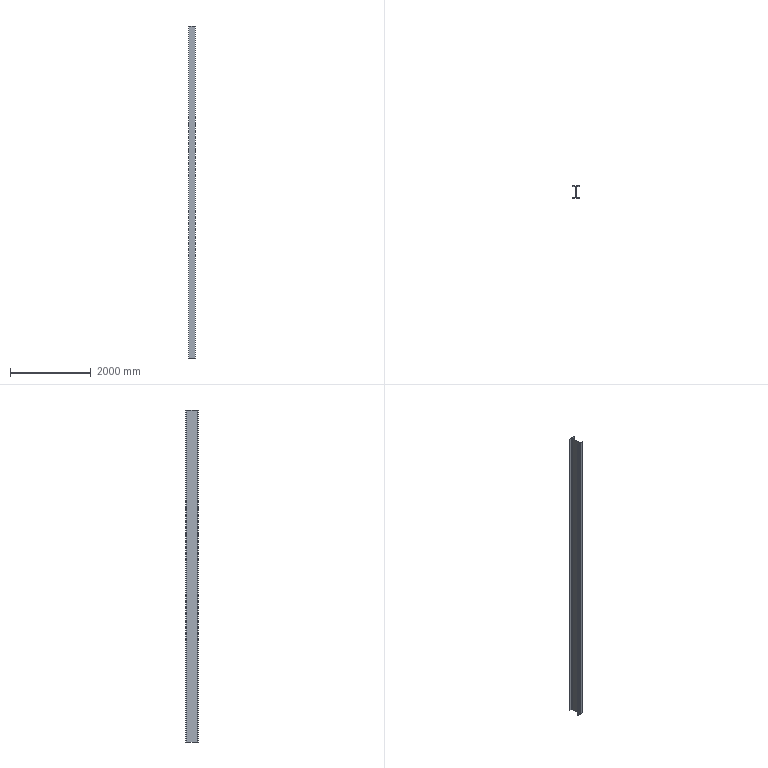Part | SolidWorks | features Extrusion 1 | 1 solid | 18 faces | box 150 x 300 x 8210 mm | volume 38406962 mm3 | plane 14 | cylinder 4 | commonest cylinder face diameters 26 x4
STEP:
#1=CARTESIAN_POINT('',(-75.,9.,0.));
#2=VERTEX_POINT('',#1);
#3=CARTESIAN_POINT('',(-75.,0.,0.));
#4=VERTEX_POINT('',#3);
#5=CARTESIAN_POINT('',(-75.,0.,0.));
#6=DIRECTION('',(0.,-1.,0.));
#7=VECTOR('',#6,1000.);
#8=LINE('',#5,#7);
#9=EDGE_CURVE('',#2,#4,#8,.T.);
#10=ORIENTED_EDGE('',*,*,#9,.T.);
#11=CARTESIAN_POINT('',(-75.,0.,8210.));
#12=VERTEX_POINT('',#11);
#13=CARTESIAN_POINT('',(-75.,0.,8210.));
#14=DIRECTION('',(0.,0.,-1.));
#15=VECTOR('',#14,1000.);
#16=LINE('',#13,#15);
#17=EDGE_CURVE('',#12,#4,#16,.T.);
#18=ORIENTED_EDGE('',*,*,#17,.F.);
#19=CARTESIAN_POINT('',(-75.,9.,8210.));
#20=VERTEX_POINT('',#19);
#21=CARTESIAN_POINT('',(-75.,0.,8210.));
#22=DIRECTION('',(0.,-1.,0.));
#23=VECTOR('',#22,1000.);
#24=LINE('',#21,#23);
#25=EDGE_CURVE('',#20,#12,#24,.T.);
#26=ORIENTED_EDGE('',*,*,#25,.F.);
#27=CARTESIAN_POINT('',(-75.,9.,8210.));
#28=DIRECTION('',(0.,0.,-1.));
#29=VECTOR('',#28,1000.);
#30=LINE('',#27,#29);
#31=EDGE_CURVE('',#20,#2,#30,.T.);
#32=ORIENTED_EDGE('',*,*,#31,.T.);
#33=EDGE_LOOP('',(#10,#18,#26,#32));
#34=FACE_OUTER_BOUND('',#33,.T.);
#35=CARTESIAN_POINT('',(-75.,0.,8210.));
#36=DIRECTION('',(1.,0.,0.));
#37=DIRECTION('',(0.,0.,-1.));
#38=AXIS2_PLACEMENT_3D('',#35,#36,#37);
#39=PLANE('',#38);
#40=ADVANCED_FACE('',(#34),#39,.F.);
#41=CARTESIAN_POINT('',(75.,0.,0.));
#42=VERTEX_POINT('',#41);
#43=CARTESIAN_POINT('',(75.,0.,0.));
#44=DIRECTION('',(1.,0.,0.));
#45=VECTOR('',#44,1000.);
#46=LINE('',#43,#45);
#47=EDGE_CURVE('',#4,#42,#46,.T.);
#48=ORIENTED_EDGE('',*,*,#47,.T.);
#49=CARTESIAN_POINT('',(75.,0.,8210.));
#50=VERTEX_POINT('',#49);
#51=CARTESIAN_POINT('',(75.,0.,8210.));
#52=DIRECTION('',(0.,0.,-1.));
#53=VECTOR('',#52,1000.);
#54=LINE('',#51,#53);
#55=EDGE_CURVE('',#50,#42,#54,.T.);
#56=ORIENTED_EDGE('',*,*,#55,.F.);
#57=CARTESIAN_POINT('',(75.,0.,8210.));
#58=DIRECTION('',(1.,0.,0.));
#59=VECTOR('',#58,1000.);
#60=LINE('',#57,#59);
#61=EDGE_CURVE('',#12,#50,#60,.T.);
#62=ORIENTED_EDGE('',*,*,#61,.F.);
#63=ORIENTED_EDGE('',*,*,#17,.T.);
#64=EDGE_LOOP('',(#48,#56,#62,#63));
#65=FACE_OUTER_BOUND('',#64,.T.);
#66=CARTESIAN_POINT('',(75.,0.,8210.));
#67=DIRECTION('',(0.,1.,0.));
#68=DIRECTION('',(-1.,0.,0.));
#69=AXIS2_PLACEMENT_3D('',#66,#67,#68);
#70=PLANE('',#69);
#71=ADVANCED_FACE('',(#65),#70,.F.);
#72=CARTESIAN_POINT('',(75.,9.,0.));
#73=VERTEX_POINT('',#72);
#74=CARTESIAN_POINT('',(75.,0.,0.));
#75=DIRECTION('',(0.,1.,0.));
#76=VECTOR('',#75,1000.);
#77=LINE('',#74,#76);
#78=EDGE_CURVE('',#42,#73,#77,.T.);
#79=ORIENTED_EDGE('',*,*,#78,.T.);
#80=CARTESIAN_POINT('',(75.,9.,8210.));
#81=VERTEX_POINT('',#80);
#82=CARTESIAN_POINT('',(75.,9.,8210.));
#83=DIRECTION('',(0.,0.,-1.));
#84=VECTOR('',#83,1000.);
#85=LINE('',#82,#84);
#86=EDGE_CURVE('',#81,#73,#85,.T.);
#87=ORIENTED_EDGE('',*,*,#86,.F.);
#88=CARTESIAN_POINT('',(75.,0.,8210.));
#89=DIRECTION('',(0.,1.,0.));
#90=VECTOR('',#89,1000.);
#91=LINE('',#88,#90);
#92=EDGE_CURVE('',#50,#81,#91,.T.);
#93=ORIENTED_EDGE('',*,*,#92,.F.);
#94=ORIENTED_EDGE('',*,*,#55,.T.);
#95=EDGE_LOOP('',(#79,#87,#93,#94));
#96=FACE_OUTER_BOUND('',#95,.T.);
#97=CARTESIAN_POINT('',(75.,0.,8210.));
#98=DIRECTION('',(-1.,0.,0.));
#99=DIRECTION('',(0.,0.,1.));
#100=AXIS2_PLACEMENT_3D('',#97,#98,#99);
#101=PLANE('',#100);
#102=ADVANCED_FACE('',(#96),#101,.F.);
#103=CARTESIAN_POINT('',(16.25,9.,0.));
#104=VERTEX_POINT('',#103);
#105=CARTESIAN_POINT('',(75.,9.,0.));
#106=DIRECTION('',(-1.,0.,0.));
#107=VECTOR('',#106,1000.);
#108=LINE('',#105,#107);
#109=EDGE_CURVE('',#73,#104,#108,.T.);
#110=ORIENTED_EDGE('',*,*,#109,.T.);
#111=CARTESIAN_POINT('',(16.25,9.,8210.));
#112=VERTEX_POINT('',#111);
#113=CARTESIAN_POINT('',(16.25,9.,8210.));
#114=DIRECTION('',(0.,0.,-1.));
#115=VECTOR('',#114,1000.);
#116=LINE('',#113,#115);
#117=EDGE_CURVE('',#112,#104,#116,.T.);
#118=ORIENTED_EDGE('',*,*,#117,.F.);
#119=CARTESIAN_POINT('',(75.,9.,8210.));
#120=DIRECTION('',(-1.,0.,0.));
#121=VECTOR('',#120,1000.);
#122=LINE('',#119,#121);
#123=EDGE_CURVE('',#81,#112,#122,.T.);
#124=ORIENTED_EDGE('',*,*,#123,.F.);
#125=ORIENTED_EDGE('',*,*,#86,.T.);
#126=EDGE_LOOP('',(#110,#118,#124,#125));
#127=FACE_OUTER_BOUND('',#126,.T.);
#128=CARTESIAN_POINT('',(75.,9.,8210.));
#129=DIRECTION('',(0.,-1.,0.));
#130=DIRECTION('',(1.,0.,0.));
#131=AXIS2_PLACEMENT_3D('',#128,#129,#130);
#132=PLANE('',#131);
#133=ADVANCED_FACE('',(#127),#132,.F.);
#134=CARTESIAN_POINT('',(3.25,22.,0.));
#135=VERTEX_POINT('',#134);
#136=CARTESIAN_POINT('',(16.25,22.,0.));
#137=DIRECTION('',(0.,0.,-1.));
#138=DIRECTION('',(-1.,0.,0.));
#139=AXIS2_PLACEMENT_3D('',#136,#137,#138);
#140=CIRCLE('',#139,13.);
#141=EDGE_CURVE('',#104,#135,#140,.T.);
#142=ORIENTED_EDGE('',*,*,#141,.T.);
#143=CARTESIAN_POINT('',(3.25,22.,8210.));
#144=VERTEX_POINT('',#143);
#145=CARTESIAN_POINT('',(3.25,22.,8210.));
#146=DIRECTION('',(0.,0.,-1.));
#147=VECTOR('',#146,1000.);
#148=LINE('',#145,#147);
#149=EDGE_CURVE('',#144,#135,#148,.T.);
#150=ORIENTED_EDGE('',*,*,#149,.F.);
#151=CARTESIAN_POINT('',(16.25,22.,8210.));
#152=DIRECTION('',(0.,0.,-1.));
#153=DIRECTION('',(-1.,0.,0.));
#154=AXIS2_PLACEMENT_3D('',#151,#152,#153);
#155=CIRCLE('',#154,13.);
#156=EDGE_CURVE('',#112,#144,#155,.T.);
#157=ORIENTED_EDGE('',*,*,#156,.F.);
#158=ORIENTED_EDGE('',*,*,#117,.T.);
#159=EDGE_LOOP('',(#142,#150,#157,#158));
#160=FACE_OUTER_BOUND('',#159,.T.);
#161=CARTESIAN_POINT('',(16.25,22.,8210.));
#162=DIRECTION('',(0.,0.,-1.));
#163=DIRECTION('',(-1.,0.,0.));
#164=AXIS2_PLACEMENT_3D('',#161,#162,#163);
#165=CYLINDRICAL_SURFACE('',#164,13.);
#166=ADVANCED_FACE('',(#160),#165,.F.);
#167=CARTESIAN_POINT('',(3.25,278.,0.));
#168=VERTEX_POINT('',#167);
#169=CARTESIAN_POINT('',(3.25,22.,0.));
#170=DIRECTION('',(0.,1.,0.));
#171=VECTOR('',#170,1000.);
#172=LINE('',#169,#171);
#173=EDGE_CURVE('',#135,#168,#172,.T.);
#174=ORIENTED_EDGE('',*,*,#173,.T.);
#175=CARTESIAN_POINT('',(3.25,278.,8210.));
#176=VERTEX_POINT('',#175);
#177=CARTESIAN_POINT('',(3.25,278.,8210.));
#178=DIRECTION('',(0.,0.,-1.));
#179=VECTOR('',#178,1000.);
#180=LINE('',#177,#179);
#181=EDGE_CURVE('',#176,#168,#180,.T.);
#182=ORIENTED_EDGE('',*,*,#181,.F.);
#183=CARTESIAN_POINT('',(3.25,22.,8210.));
#184=DIRECTION('',(0.,1.,0.));
#185=VECTOR('',#184,1000.);
#186=LINE('',#183,#185);
#187=EDGE_CURVE('',#144,#176,#186,.T.);
#188=ORIENTED_EDGE('',*,*,#187,.F.);
#189=ORIENTED_EDGE('',*,*,#149,.T.);
#190=EDGE_LOOP('',(#174,#182,#188,#189));
#191=FACE_OUTER_BOUND('',#190,.T.);
#192=CARTESIAN_POINT('',(3.25,22.,8210.));
#193=DIRECTION('',(-1.,0.,0.));
#194=DIRECTION('',(0.,0.,1.));
#195=AXIS2_PLACEMENT_3D('',#192,#193,#194);
#196=PLANE('',#195);
#197=ADVANCED_FACE('',(#191),#196,.F.);
#198=CARTESIAN_POINT('',(16.25,291.,0.));
#199=VERTEX_POINT('',#198);
#200=CARTESIAN_POINT('',(16.25,278.,0.));
#201=DIRECTION('',(0.,0.,-1.));
#202=DIRECTION('',(-1.,0.,0.));
#203=AXIS2_PLACEMENT_3D('',#200,#201,#202);
#204=CIRCLE('',#203,13.);
#205=EDGE_CURVE('',#168,#199,#204,.T.);
#206=ORIENTED_EDGE('',*,*,#205,.T.);
#207=CARTESIAN_POINT('',(16.25,291.,8210.));
#208=VERTEX_POINT('',#207);
#209=CARTESIAN_POINT('',(16.25,291.,8210.));
#210=DIRECTION('',(0.,0.,-1.));
#211=VECTOR('',#210,1000.);
#212=LINE('',#209,#211);
#213=EDGE_CURVE('',#208,#199,#212,.T.);
#214=ORIENTED_EDGE('',*,*,#213,.F.);
#215=CARTESIAN_POINT('',(16.25,278.,8210.));
#216=DIRECTION('',(0.,0.,-1.));
#217=DIRECTION('',(-1.,0.,0.));
#218=AXIS2_PLACEMENT_3D('',#215,#216,#217);
#219=CIRCLE('',#218,13.);
#220=EDGE_CURVE('',#176,#208,#219,.T.);
#221=ORIENTED_EDGE('',*,*,#220,.F.);
#222=ORIENTED_EDGE('',*,*,#181,.T.);
#223=EDGE_LOOP('',(#206,#214,#221,#222));
#224=FACE_OUTER_BOUND('',#223,.T.);
#225=CARTESIAN_POINT('',(16.25,278.,8210.));
#226=DIRECTION('',(0.,0.,-1.));
#227=DIRECTION('',(-1.,0.,0.));
#228=AXIS2_PLACEMENT_3D('',#225,#226,#227);
#229=CYLINDRICAL_SURFACE('',#228,13.);
#230=ADVANCED_FACE('',(#224),#229,.F.);
#231=CARTESIAN_POINT('',(75.,291.,0.));
#232=VERTEX_POINT('',#231);
#233=CARTESIAN_POINT('',(16.25,291.,0.));
#234=DIRECTION('',(1.,0.,0.));
#235=VECTOR('',#234,1000.);
#236=LINE('',#233,#235);
#237=EDGE_CURVE('',#199,#232,#236,.T.);
#238=ORIENTED_EDGE('',*,*,#237,.T.);
#239=CARTESIAN_POINT('',(75.,291.,8210.));
#240=VERTEX_POINT('',#239);
#241=CARTESIAN_POINT('',(75.,291.,8210.));
#242=DIRECTION('',(0.,0.,-1.));
#243=VECTOR('',#242,1000.);
#244=LINE('',#241,#243);
#245=EDGE_CURVE('',#240,#232,#244,.T.);
#246=ORIENTED_EDGE('',*,*,#245,.F.);
#247=CARTESIAN_POINT('',(16.25,291.,8210.));
#248=DIRECTION('',(1.,0.,0.));
#249=VECTOR('',#248,1000.);
#250=LINE('',#247,#249);
#251=EDGE_CURVE('',#208,#240,#250,.T.);
#252=ORIENTED_EDGE('',*,*,#251,.F.);
#253=ORIENTED_EDGE('',*,*,#213,.T.);
#254=EDGE_LOOP('',(#238,#246,#252,#253));
#255=FACE_OUTER_BOUND('',#254,.T.);
#256=CARTESIAN_POINT('',(16.25,291.,8210.));
#257=DIRECTION('',(0.,1.,0.));
#258=DIRECTION('',(-1.,0.,0.));
#259=AXIS2_PLACEMENT_3D('',#256,#257,#258);
#260=PLANE('',#259);
#261=ADVANCED_FACE('',(#255),#260,.F.);
#262=CARTESIAN_POINT('',(75.,300.,0.));
#263=VERTEX_POINT('',#262);
#264=CARTESIAN_POINT('',(75.,291.,0.));
#265=DIRECTION('',(0.,1.,0.));
#266=VECTOR('',#265,1000.);
#267=LINE('',#264,#266);
#268=EDGE_CURVE('',#232,#263,#267,.T.);
#269=ORIENTED_EDGE('',*,*,#268,.T.);
#270=CARTESIAN_POINT('',(75.,300.,8210.));
#271=VERTEX_POINT('',#270);
#272=CARTESIAN_POINT('',(75.,300.,8210.));
#273=DIRECTION('',(0.,0.,-1.));
#274=VECTOR('',#273,1000.);
#275=LINE('',#272,#274);
#276=EDGE_CURVE('',#271,#263,#275,.T.);
#277=ORIENTED_EDGE('',*,*,#276,.F.);
#278=CARTESIAN_POINT('',(75.,291.,8210.));
#279=DIRECTION('',(0.,1.,0.));
#280=VECTOR('',#279,1000.);
#281=LINE('',#278,#280);
#282=EDGE_CURVE('',#240,#271,#281,.T.);
#283=ORIENTED_EDGE('',*,*,#282,.F.);
#284=ORIENTED_EDGE('',*,*,#245,.T.);
#285=EDGE_LOOP('',(#269,#277,#283,#284));
#286=FACE_OUTER_BOUND('',#285,.T.);
#287=CARTESIAN_POINT('',(75.,291.,8210.));
#288=DIRECTION('',(-1.,0.,0.));
#289=DIRECTION('',(0.,-1.,0.));
#290=AXIS2_PLACEMENT_3D('',#287,#288,#289);
#291=PLANE('',#290);
#292=ADVANCED_FACE('',(#286),#291,.F.);
#293=CARTESIAN_POINT('',(-75.,300.,0.));
#294=VERTEX_POINT('',#293);
#295=CARTESIAN_POINT('',(-75.,300.,0.));
#296=DIRECTION('',(-1.,0.,0.));
#297=VECTOR('',#296,1000.);
#298=LINE('',#295,#297);
#299=EDGE_CURVE('',#263,#294,#298,.T.);
#300=ORIENTED_EDGE('',*,*,#299,.T.);
#301=CARTESIAN_POINT('',(-75.,300.,8210.));
#302=VERTEX_POINT('',#301);
#303=CARTESIAN_POINT('',(-75.,300.,8210.));
#304=DIRECTION('',(0.,0.,-1.));
#305=VECTOR('',#304,1000.);
#306=LINE('',#303,#305);
#307=EDGE_CURVE('',#302,#294,#306,.T.);
#308=ORIENTED_EDGE('',*,*,#307,.F.);
#309=CARTESIAN_POINT('',(-75.,300.,8210.));
#310=DIRECTION('',(-1.,0.,0.));
#311=VECTOR('',#310,1000.);
#312=LINE('',#309,#311);
#313=EDGE_CURVE('',#271,#302,#312,.T.);
#314=ORIENTED_EDGE('',*,*,#313,.F.);
#315=ORIENTED_EDGE('',*,*,#276,.T.);
#316=EDGE_LOOP('',(#300,#308,#314,#315));
#317=FACE_OUTER_BOUND('',#316,.T.);
#318=CARTESIAN_POINT('',(-75.,300.,8210.));
#319=DIRECTION('',(0.,-1.,0.));
#320=DIRECTION('',(0.,0.,-1.));
#321=AXIS2_PLACEMENT_3D('',#318,#319,#320);
#322=PLANE('',#321);
#323=ADVANCED_FACE('',(#317),#322,.F.);
#324=CARTESIAN_POINT('',(-75.,291.,0.));
#325=VERTEX_POINT('',#324);
#326=CARTESIAN_POINT('',(-75.,291.,0.));
#327=DIRECTION('',(0.,-1.,0.));
#328=VECTOR('',#327,1000.);
#329=LINE('',#326,#328);
#330=EDGE_CURVE('',#294,#325,#329,.T.);
#331=ORIENTED_EDGE('',*,*,#330,.T.);
#332=CARTESIAN_POINT('',(-75.,291.,8210.));
#333=VERTEX_POINT('',#332);
#334=CARTESIAN_POINT('',(-75.,291.,8210.));
#335=DIRECTION('',(0.,0.,-1.));
#336=VECTOR('',#335,1000.);
#337=LINE('',#334,#336);
#338=EDGE_CURVE('',#333,#325,#337,.T.);
#339=ORIENTED_EDGE('',*,*,#338,.F.);
#340=CARTESIAN_POINT('',(-75.,291.,8210.));
#341=DIRECTION('',(0.,-1.,0.));
#342=VECTOR('',#341,1000.);
#343=LINE('',#340,#342);
#344=EDGE_CURVE('',#302,#333,#343,.T.);
#345=ORIENTED_EDGE('',*,*,#344,.F.);
#346=ORIENTED_EDGE('',*,*,#307,.T.);
#347=EDGE_LOOP('',(#331,#339,#345,#346));
#348=FACE_OUTER_BOUND('',#347,.T.);
#349=CARTESIAN_POINT('',(-75.,291.,8210.));
#350=DIRECTION('',(1.,0.,0.));
#351=DIRECTION('',(0.,1.,0.));
#352=AXIS2_PLACEMENT_3D('',#349,#350,#351);
#353=PLANE('',#352);
#354=ADVANCED_FACE('',(#348),#353,.F.);
#355=CARTESIAN_POINT('',(-16.25,291.,0.));
#356=VERTEX_POINT('',#355);
#357=CARTESIAN_POINT('',(-16.25,291.,0.));
#358=DIRECTION('',(1.,0.,0.));
#359=VECTOR('',#358,1000.);
#360=LINE('',#357,#359);
#361=EDGE_CURVE('',#325,#356,#360,.T.);
#362=ORIENTED_EDGE('',*,*,#361,.T.);
#363=CARTESIAN_POINT('',(-16.25,291.,8210.));
#364=VERTEX_POINT('',#363);
#365=CARTESIAN_POINT('',(-16.25,291.,8210.));
#366=DIRECTION('',(0.,0.,-1.));
#367=VECTOR('',#366,1000.);
#368=LINE('',#365,#367);
#369=EDGE_CURVE('',#364,#356,#368,.T.);
#370=ORIENTED_EDGE('',*,*,#369,.F.);
#371=CARTESIAN_POINT('',(-16.25,291.,8210.));
#372=DIRECTION('',(1.,0.,0.));
#373=VECTOR('',#372,1000.);
#374=LINE('',#371,#373);
#375=EDGE_CURVE('',#333,#364,#374,.T.);
#376=ORIENTED_EDGE('',*,*,#375,.F.);
#377=ORIENTED_EDGE('',*,*,#338,.T.);
#378=EDGE_LOOP('',(#362,#370,#376,#377));
#379=FACE_OUTER_BOUND('',#378,.T.);
#380=CARTESIAN_POINT('',(-16.25,291.,8210.));
#381=DIRECTION('',(0.,1.,0.));
#382=DIRECTION('',(-1.,0.,0.));
#383=AXIS2_PLACEMENT_3D('',#380,#381,#382);
#384=PLANE('',#383);
#385=ADVANCED_FACE('',(#379),#384,.F.);
#386=CARTESIAN_POINT('',(-3.25,278.,0.));
#387=VERTEX_POINT('',#386);
#388=CARTESIAN_POINT('',(-16.25,278.,0.));
#389=DIRECTION('',(0.,0.,-1.));
#390=DIRECTION('',(1.,0.,0.));
#391=AXIS2_PLACEMENT_3D('',#388,#389,#390);
#392=CIRCLE('',#391,13.);
#393=EDGE_CURVE('',#356,#387,#392,.T.);
#394=ORIENTED_EDGE('',*,*,#393,.T.);
#395=CARTESIAN_POINT('',(-3.25,278.,8210.));
#396=VERTEX_POINT('',#395);
#397=CARTESIAN_POINT('',(-3.25,278.,8210.));
#398=DIRECTION('',(0.,0.,-1.));
#399=VECTOR('',#398,1000.);
#400=LINE('',#397,#399);
#401=EDGE_CURVE('',#396,#387,#400,.T.);
#402=ORIENTED_EDGE('',*,*,#401,.F.);
#403=CARTESIAN_POINT('',(-16.25,278.,8210.));
#404=DIRECTION('',(0.,0.,-1.));
#405=DIRECTION('',(1.,0.,0.));
#406=AXIS2_PLACEMENT_3D('',#403,#404,#405);
#407=CIRCLE('',#406,13.);
#408=EDGE_CURVE('',#364,#396,#407,.T.);
#409=ORIENTED_EDGE('',*,*,#408,.F.);
#410=ORIENTED_EDGE('',*,*,#369,.T.);
#411=EDGE_LOOP('',(#394,#402,#409,#410));
#412=FACE_OUTER_BOUND('',#411,.T.);
#413=CARTESIAN_POINT('',(-16.25,278.,8210.));
#414=DIRECTION('',(0.,0.,-1.));
#415=DIRECTION('',(-1.,0.,0.));
#416=AXIS2_PLACEMENT_3D('',#413,#414,#415);
#417=CYLINDRICAL_SURFACE('',#416,13.);
#418=ADVANCED_FACE('',(#412),#417,.F.);
#419=CARTESIAN_POINT('',(-3.25,22.,0.));
#420=VERTEX_POINT('',#419);
#421=CARTESIAN_POINT('',(-3.25,22.,0.));
#422=DIRECTION('',(0.,-1.,0.));
#423=VECTOR('',#422,1000.);
#424=LINE('',#421,#423);
#425=EDGE_CURVE('',#387,#420,#424,.T.);
#426=ORIENTED_EDGE('',*,*,#425,.T.);
#427=CARTESIAN_POINT('',(-3.25,22.,8210.));
#428=VERTEX_POINT('',#427);
#429=CARTESIAN_POINT('',(-3.25,22.,8210.));
#430=DIRECTION('',(0.,0.,-1.));
#431=VECTOR('',#430,1000.);
#432=LINE('',#429,#431);
#433=EDGE_CURVE('',#428,#420,#432,.T.);
#434=ORIENTED_EDGE('',*,*,#433,.F.);
#435=CARTESIAN_POINT('',(-3.25,22.,8210.));
#436=DIRECTION('',(0.,-1.,0.));
#437=VECTOR('',#436,1000.);
#438=LINE('',#435,#437);
#439=EDGE_CURVE('',#396,#428,#438,.T.);
#440=ORIENTED_EDGE('',*,*,#439,.F.);
#441=ORIENTED_EDGE('',*,*,#401,.T.);
#442=EDGE_LOOP('',(#426,#434,#440,#441));
#443=FACE_OUTER_BOUND('',#442,.T.);
#444=CARTESIAN_POINT('',(-3.25,22.,8210.));
#445=DIRECTION('',(1.,0.,0.));
#446=DIRECTION('',(0.,0.,-1.));
#447=AXIS2_PLACEMENT_3D('',#444,#445,#446);
#448=PLANE('',#447);
#449=ADVANCED_FACE('',(#443),#448,.F.);
#450=CARTESIAN_POINT('',(-16.25,9.,0.));
#451=VERTEX_POINT('',#450);
#452=CARTESIAN_POINT('',(-16.25,22.,0.));
#453=DIRECTION('',(0.,0.,-1.));
#454=DIRECTION('',(-1.,0.,0.));
#455=AXIS2_PLACEMENT_3D('',#452,#453,#454);
#456=CIRCLE('',#455,13.);
#457=EDGE_CURVE('',#420,#451,#456,.T.);
#458=ORIENTED_EDGE('',*,*,#457,.T.);
#459=CARTESIAN_POINT('',(-16.25,9.,8210.));
#460=VERTEX_POINT('',#459);
#461=CARTESIAN_POINT('',(-16.25,9.,8210.));
#462=DIRECTION('',(0.,0.,-1.));
#463=VECTOR('',#462,1000.);
#464=LINE('',#461,#463);
#465=EDGE_CURVE('',#460,#451,#464,.T.);
#466=ORIENTED_EDGE('',*,*,#465,.F.);
#467=CARTESIAN_POINT('',(-16.25,22.,8210.));
#468=DIRECTION('',(0.,0.,-1.));
#469=DIRECTION('',(-1.,0.,0.));
#470=AXIS2_PLACEMENT_3D('',#467,#468,#469);
#471=CIRCLE('',#470,13.);
#472=EDGE_CURVE('',#428,#460,#471,.T.);
#473=ORIENTED_EDGE('',*,*,#472,.F.);
#474=ORIENTED_EDGE('',*,*,#433,.T.);
#475=EDGE_LOOP('',(#458,#466,#473,#474));
#476=FACE_OUTER_BOUND('',#475,.T.);
#477=CARTESIAN_POINT('',(-16.25,22.,8210.));
#478=DIRECTION('',(0.,0.,-1.));
#479=DIRECTION('',(-1.,0.,0.));
#480=AXIS2_PLACEMENT_3D('',#477,#478,#479);
#481=CYLINDRICAL_SURFACE('',#480,13.);
#482=ADVANCED_FACE('',(#476),#481,.F.);
#483=CARTESIAN_POINT('',(-75.,9.,0.));
#484=DIRECTION('',(-1.,0.,0.));
#485=VECTOR('',#484,1000.);
#486=LINE('',#483,#485);
#487=EDGE_CURVE('',#451,#2,#486,.T.);
#488=ORIENTED_EDGE('',*,*,#487,.T.);
#489=ORIENTED_EDGE('',*,*,#31,.F.);
#490=CARTESIAN_POINT('',(-75.,9.,8210.));
#491=DIRECTION('',(-1.,0.,0.));
#492=VECTOR('',#491,1000.);
#493=LINE('',#490,#492);
#494=EDGE_CURVE('',#460,#20,#493,.T.);
#495=ORIENTED_EDGE('',*,*,#494,.F.);
#496=ORIENTED_EDGE('',*,*,#465,.T.);
#497=EDGE_LOOP('',(#488,#489,#495,#496));
#498=FACE_OUTER_BOUND('',#497,.T.);
#499=CARTESIAN_POINT('',(-75.,9.,8210.));
#500=DIRECTION('',(0.,-1.,0.));
#501=DIRECTION('',(1.,0.,0.));
#502=AXIS2_PLACEMENT_3D('',#499,#500,#501);
#503=PLANE('',#502);
#504=ADVANCED_FACE('',(#498),#503,.F.);
#505=ORIENTED_EDGE('',*,*,#25,.T.);
#506=ORIENTED_EDGE('',*,*,#61,.T.);
#507=ORIENTED_EDGE('',*,*,#92,.T.);
#508=ORIENTED_EDGE('',*,*,#123,.T.);
#509=ORIENTED_EDGE('',*,*,#156,.T.);
#510=ORIENTED_EDGE('',*,*,#187,.T.);
#511=ORIENTED_EDGE('',*,*,#220,.T.);
#512=ORIENTED_EDGE('',*,*,#251,.T.);
#513=ORIENTED_EDGE('',*,*,#282,.T.);
#514=ORIENTED_EDGE('',*,*,#313,.T.);
#515=ORIENTED_EDGE('',*,*,#344,.T.);
#516=ORIENTED_EDGE('',*,*,#375,.T.);
#517=ORIENTED_EDGE('',*,*,#408,.T.);
#518=ORIENTED_EDGE('',*,*,#439,.T.);
#519=ORIENTED_EDGE('',*,*,#472,.T.);
#520=ORIENTED_EDGE('',*,*,#494,.T.);
#521=EDGE_LOOP('',(#505,#506,#507,#508,#509,#510,#511,#512,#513,#514,#515,#516,#517,#518,#519,#520));
#522=FACE_OUTER_BOUND('',#521,.T.);
#523=CARTESIAN_POINT('',(-16.25,22.,8210.));
#524=DIRECTION('',(0.,0.,-1.));
#525=DIRECTION('',(-1.,0.,0.));
#526=AXIS2_PLACEMENT_3D('',#523,#524,#525);
#527=PLANE('',#526);
#528=ADVANCED_FACE('',(#522),#527,.F.);
#529=ORIENTED_EDGE('',*,*,#9,.F.);
#530=ORIENTED_EDGE('',*,*,#487,.F.);
#531=ORIENTED_EDGE('',*,*,#457,.F.);
#532=ORIENTED_EDGE('',*,*,#425,.F.);
#533=ORIENTED_EDGE('',*,*,#393,.F.);
#534=ORIENTED_EDGE('',*,*,#361,.F.);
#535=ORIENTED_EDGE('',*,*,#330,.F.);
#536=ORIENTED_EDGE('',*,*,#299,.F.);
#537=ORIENTED_EDGE('',*,*,#268,.F.);
#538=ORIENTED_EDGE('',*,*,#237,.F.);
#539=ORIENTED_EDGE('',*,*,#205,.F.);
#540=ORIENTED_EDGE('',*,*,#173,.F.);
#541=ORIENTED_EDGE('',*,*,#141,.F.);
#542=ORIENTED_EDGE('',*,*,#109,.F.);
#543=ORIENTED_EDGE('',*,*,#78,.F.);
#544=ORIENTED_EDGE('',*,*,#47,.F.);
#545=EDGE_LOOP('',(#529,#530,#531,#532,#533,#534,#535,#536,#537,#538,#539,#540,#541,#542,#543,#544));
#546=FACE_OUTER_BOUND('',#545,.T.);
#547=CARTESIAN_POINT('',(-16.25,22.,0.));
#548=DIRECTION('',(0.,0.,-1.));
#549=DIRECTION('',(-1.,0.,0.));
#550=AXIS2_PLACEMENT_3D('',#547,#548,#549);
#551=PLANE('',#550);
#552=ADVANCED_FACE('',(#546),#551,.T.);
#553=CLOSED_SHELL('',(#40,#71,#102,#133,#166,#197,#230,#261,#292,#323,#354,#385,#418,#449,#482,#504,#528,#552));
#554=MANIFOLD_SOLID_BREP('',#553);
#555=CARTESIAN_POINT('',(0.,0.,0.));
#556=DIRECTION('',(0.,0.,1.));
#557=DIRECTION('',(1.,0.,0.));
#558=AXIS2_PLACEMENT_3D('',#555,#556,#557);
#559=(LENGTH_UNIT()NAMED_UNIT(*)SI_UNIT(.MILLI.,.METRE.));
#560=UNCERTAINTY_MEASURE_WITH_UNIT(LENGTH_MEASURE(0.00001),#559,'','');
#561=(NAMED_UNIT(*)PLANE_ANGLE_UNIT()SI_UNIT($,.RADIAN.));
#562=(NAMED_UNIT(*)SI_UNIT($,.STERADIAN.)SOLID_ANGLE_UNIT());
#563=(GEOMETRIC_REPRESENTATION_CONTEXT(3)GLOBAL_UNCERTAINTY_ASSIGNED_CONTEXT((#560))GLOBAL_UNIT_ASSIGNED_CONTEXT((#559,#561,#562))REPRESENTATION_CONTEXT('',''));
#564=ADVANCED_BREP_SHAPE_REPRESENTATION('',(#554,#558),#563);